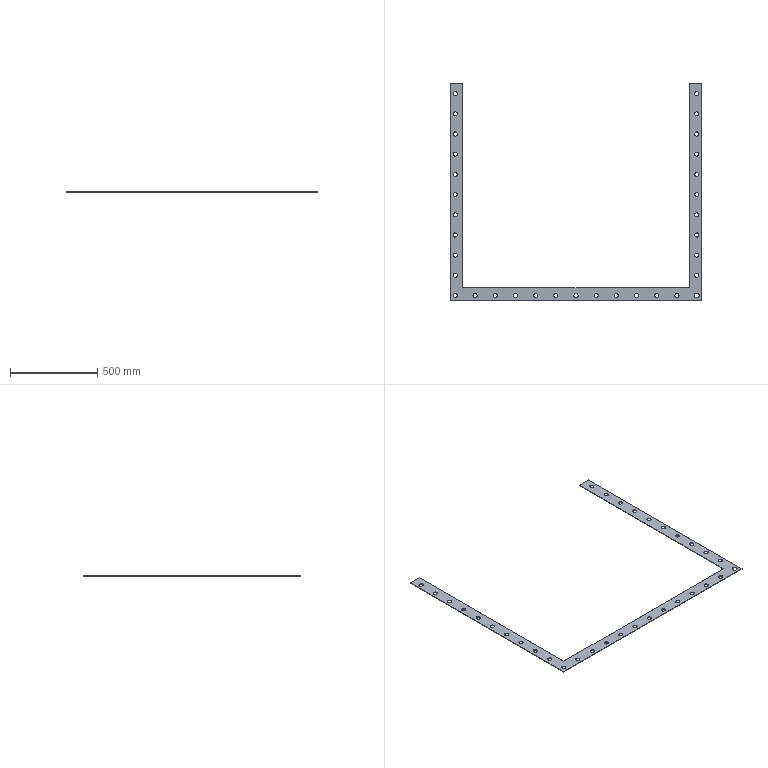Part | SolidWorks | features Extrusion 1 | 1 solid | 76 faces | box 1448 x 1250 x 3 mm | volume 798363 mm3 | cylinder 66 | plane 10 | commonest cylinder face diameters 24 x64 27.698 x2